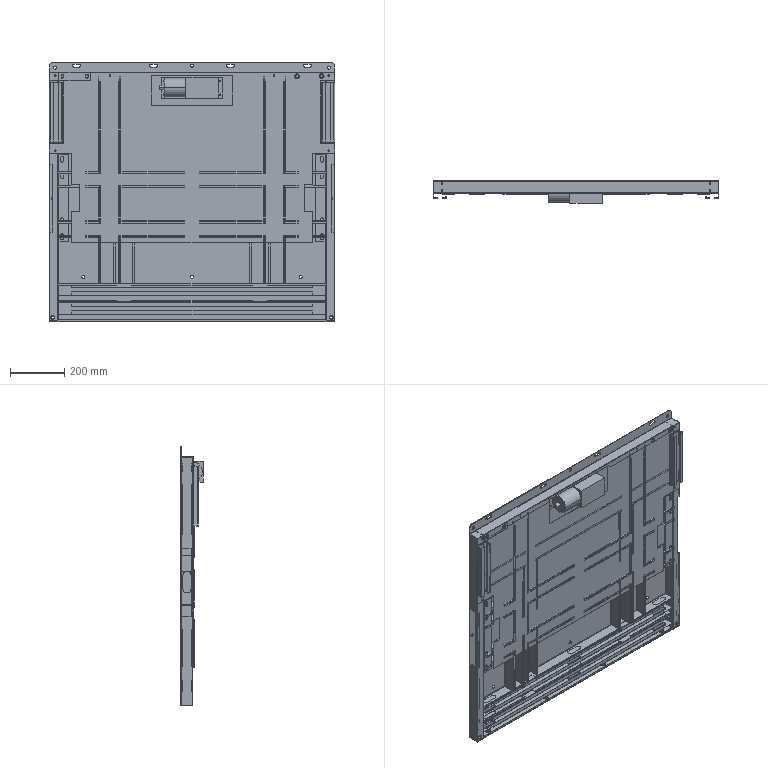Part | 34 solids | 2063 faces | box 1050 x 81.5 x 955 mm | volume 5936154 mm3 | plane 1524 | cylinder 515 | cone 24 | commonest cylinder face diameters 0.4 x118 3.4 x100 10 x92 20 x38 5 x20 6 x20